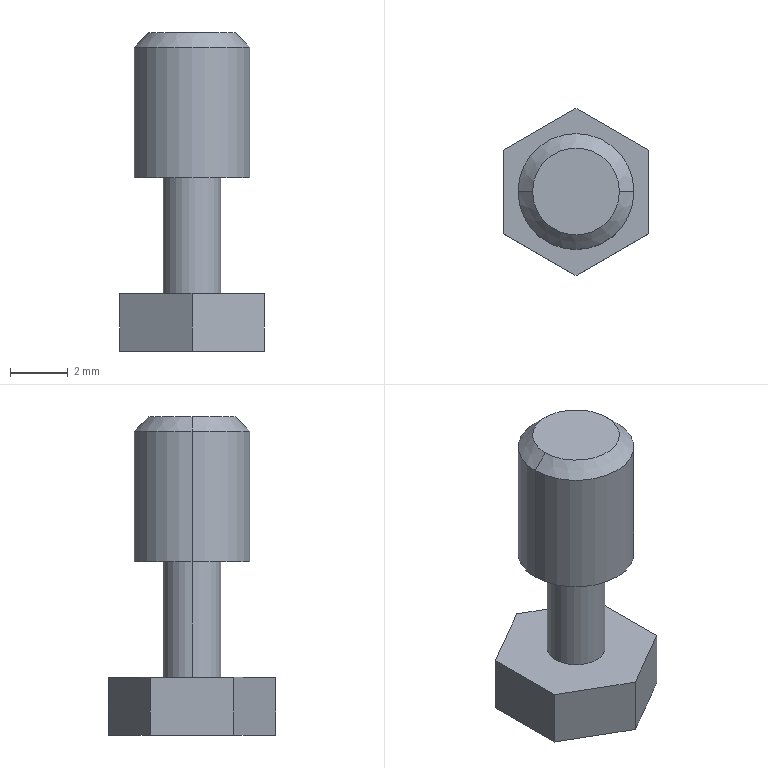Part | SolidWorks | features ICE 2, Chamfer 1, Extrusion 1 | 1 solid | 16 faces | box 5 x 5.774 x 11 mm | volume 117.26 mm3 | plane 10 | cylinder 4 | cone 2 | commonest cylinder face diameters 2 x2 4 x2
STEP:
#1=CARTESIAN_POINT('',(1.5,0.,5.));
#2=VERTEX_POINT('',#1);
#3=CARTESIAN_POINT('',(-1.5,0.,5.));
#4=VERTEX_POINT('',#3);
#5=CARTESIAN_POINT('',(0.,0.,5.));
#6=DIRECTION('',(0.,0.,1.));
#7=DIRECTION('',(1.,0.,0.));
#8=AXIS2_PLACEMENT_3D('',#5,#6,#7);
#9=CIRCLE('',#8,1.5);
#10=EDGE_CURVE('',#2,#4,#9,.T.);
#11=ORIENTED_EDGE('',*,*,#10,.F.);
#12=CARTESIAN_POINT('',(2.,0.,4.5));
#13=VERTEX_POINT('',#12);
#14=CARTESIAN_POINT('',(1.5,0.,5.));
#15=DIRECTION('',(0.7071,0.,-0.7071));
#16=VECTOR('',#15,1000.);
#17=LINE('',#14,#16);
#18=EDGE_CURVE('',#2,#13,#17,.T.);
#19=ORIENTED_EDGE('',*,*,#18,.T.);
#20=CARTESIAN_POINT('',(-2.,0.,4.5));
#21=VERTEX_POINT('',#20);
#22=CARTESIAN_POINT('',(0.,0.,4.5));
#23=DIRECTION('',(0.,0.,-1.));
#24=DIRECTION('',(1.,0.,0.));
#25=AXIS2_PLACEMENT_3D('',#22,#23,#24);
#26=CIRCLE('',#25,2.);
#27=EDGE_CURVE('',#21,#13,#26,.T.);
#28=ORIENTED_EDGE('',*,*,#27,.F.);
#29=CARTESIAN_POINT('',(-1.5,0.,5.));
#30=DIRECTION('',(-0.7071,0.,-0.7071));
#31=VECTOR('',#30,1000.);
#32=LINE('',#29,#31);
#33=EDGE_CURVE('',#4,#21,#32,.T.);
#34=ORIENTED_EDGE('',*,*,#33,.F.);
#35=EDGE_LOOP('',(#11,#19,#28,#34));
#36=FACE_OUTER_BOUND('',#35,.T.);
#37=CARTESIAN_POINT('',(0.,0.,5.));
#38=DIRECTION('',(0.,0.,-1.));
#39=DIRECTION('',(-1.,0.,0.));
#40=AXIS2_PLACEMENT_3D('',#37,#38,#39);
#41=CONICAL_SURFACE('',#40,1.5,0.7854);
#42=ADVANCED_FACE('',(#36),#41,.T.);
#43=CARTESIAN_POINT('',(-1.,0.,-4.));
#44=VERTEX_POINT('',#43);
#45=CARTESIAN_POINT('',(1.,0.,-4.));
#46=VERTEX_POINT('',#45);
#47=CARTESIAN_POINT('',(0.,0.,-4.));
#48=DIRECTION('',(0.,0.,-1.));
#49=DIRECTION('',(-1.,0.,0.));
#50=AXIS2_PLACEMENT_3D('',#47,#48,#49);
#51=CIRCLE('',#50,1.);
#52=EDGE_CURVE('',#44,#46,#51,.T.);
#53=ORIENTED_EDGE('',*,*,#52,.F.);
#54=CARTESIAN_POINT('',(-1.,0.,0.));
#55=VERTEX_POINT('',#54);
#56=CARTESIAN_POINT('',(-1.,0.,-4.));
#57=DIRECTION('',(0.,0.,1.));
#58=VECTOR('',#57,1000.);
#59=LINE('',#56,#58);
#60=EDGE_CURVE('',#44,#55,#59,.T.);
#61=ORIENTED_EDGE('',*,*,#60,.T.);
#62=CARTESIAN_POINT('',(1.,0.,0.));
#63=VERTEX_POINT('',#62);
#64=CARTESIAN_POINT('',(0.,0.,0.));
#65=DIRECTION('',(0.,0.,-1.));
#66=DIRECTION('',(-1.,0.,0.));
#67=AXIS2_PLACEMENT_3D('',#64,#65,#66);
#68=CIRCLE('',#67,1.);
#69=EDGE_CURVE('',#55,#63,#68,.T.);
#70=ORIENTED_EDGE('',*,*,#69,.T.);
#71=CARTESIAN_POINT('',(1.,0.,-4.));
#72=DIRECTION('',(0.,0.,1.));
#73=VECTOR('',#72,1000.);
#74=LINE('',#71,#73);
#75=EDGE_CURVE('',#46,#63,#74,.T.);
#76=ORIENTED_EDGE('',*,*,#75,.F.);
#77=EDGE_LOOP('',(#53,#61,#70,#76));
#78=FACE_OUTER_BOUND('',#77,.T.);
#79=CARTESIAN_POINT('',(0.,0.,-4.));
#80=DIRECTION('',(0.,0.,1.));
#81=DIRECTION('',(1.,0.,0.));
#82=AXIS2_PLACEMENT_3D('',#79,#80,#81);
#83=CYLINDRICAL_SURFACE('',#82,1.);
#84=ADVANCED_FACE('',(#78),#83,.T.);
#85=ORIENTED_EDGE('',*,*,#27,.T.);
#86=CARTESIAN_POINT('',(2.,0.,0.));
#87=VERTEX_POINT('',#86);
#88=CARTESIAN_POINT('',(2.,0.,5.));
#89=DIRECTION('',(0.,0.,-1.));
#90=VECTOR('',#89,1000.);
#91=LINE('',#88,#90);
#92=EDGE_CURVE('',#13,#87,#91,.T.);
#93=ORIENTED_EDGE('',*,*,#92,.T.);
#94=CARTESIAN_POINT('',(-2.,0.,0.));
#95=VERTEX_POINT('',#94);
#96=CARTESIAN_POINT('',(0.,0.,0.));
#97=DIRECTION('',(0.,0.,1.));
#98=DIRECTION('',(1.,0.,0.));
#99=AXIS2_PLACEMENT_3D('',#96,#97,#98);
#100=CIRCLE('',#99,2.);
#101=EDGE_CURVE('',#87,#95,#100,.T.);
#102=ORIENTED_EDGE('',*,*,#101,.T.);
#103=CARTESIAN_POINT('',(-2.,0.,5.));
#104=DIRECTION('',(0.,0.,-1.));
#105=VECTOR('',#104,1000.);
#106=LINE('',#103,#105);
#107=EDGE_CURVE('',#21,#95,#106,.T.);
#108=ORIENTED_EDGE('',*,*,#107,.F.);
#109=EDGE_LOOP('',(#85,#93,#102,#108));
#110=FACE_OUTER_BOUND('',#109,.T.);
#111=CARTESIAN_POINT('',(0.,0.,5.));
#112=DIRECTION('',(0.,0.,-1.));
#113=DIRECTION('',(-1.,0.,0.));
#114=AXIS2_PLACEMENT_3D('',#111,#112,#113);
#115=CYLINDRICAL_SURFACE('',#114,2.);
#116=ADVANCED_FACE('',(#110),#115,.T.);
#117=ORIENTED_EDGE('',*,*,#92,.F.);
#118=CARTESIAN_POINT('',(0.,0.,4.5));
#119=DIRECTION('',(0.,0.,-1.));
#120=DIRECTION('',(1.,0.,0.));
#121=AXIS2_PLACEMENT_3D('',#118,#119,#120);
#122=CIRCLE('',#121,2.);
#123=EDGE_CURVE('',#13,#21,#122,.T.);
#124=ORIENTED_EDGE('',*,*,#123,.T.);
#125=ORIENTED_EDGE('',*,*,#107,.T.);
#126=CARTESIAN_POINT('',(0.,0.,0.));
#127=DIRECTION('',(0.,0.,1.));
#128=DIRECTION('',(1.,0.,0.));
#129=AXIS2_PLACEMENT_3D('',#126,#127,#128);
#130=CIRCLE('',#129,2.);
#131=EDGE_CURVE('',#95,#87,#130,.T.);
#132=ORIENTED_EDGE('',*,*,#131,.T.);
#133=EDGE_LOOP('',(#117,#124,#125,#132));
#134=FACE_OUTER_BOUND('',#133,.T.);
#135=CARTESIAN_POINT('',(0.,0.,5.));
#136=DIRECTION('',(0.,0.,-1.));
#137=DIRECTION('',(-1.,0.,0.));
#138=AXIS2_PLACEMENT_3D('',#135,#136,#137);
#139=CYLINDRICAL_SURFACE('',#138,2.);
#140=ADVANCED_FACE('',(#134),#139,.T.);
#141=CARTESIAN_POINT('',(0.,0.,5.));
#142=DIRECTION('',(0.,0.,1.));
#143=DIRECTION('',(1.,0.,0.));
#144=AXIS2_PLACEMENT_3D('',#141,#142,#143);
#145=CIRCLE('',#144,1.5);
#146=EDGE_CURVE('',#4,#2,#145,.T.);
#147=ORIENTED_EDGE('',*,*,#146,.T.);
#148=ORIENTED_EDGE('',*,*,#10,.T.);
#149=EDGE_LOOP('',(#147,#148));
#150=FACE_OUTER_BOUND('',#149,.T.);
#151=CARTESIAN_POINT('',(0.,0.,5.));
#152=DIRECTION('',(0.,0.,1.));
#153=DIRECTION('',(1.,0.,0.));
#154=AXIS2_PLACEMENT_3D('',#151,#152,#153);
#155=PLANE('',#154);
#156=ADVANCED_FACE('',(#150),#155,.T.);
#157=CARTESIAN_POINT('',(0.,0.,0.));
#158=DIRECTION('',(0.,0.,-1.));
#159=DIRECTION('',(-1.,0.,0.));
#160=AXIS2_PLACEMENT_3D('',#157,#158,#159);
#161=CIRCLE('',#160,1.);
#162=EDGE_CURVE('',#63,#55,#161,.T.);
#163=ORIENTED_EDGE('',*,*,#162,.F.);
#164=ORIENTED_EDGE('',*,*,#69,.F.);
#165=EDGE_LOOP('',(#163,#164));
#166=FACE_BOUND('',#165,.T.);
#167=ORIENTED_EDGE('',*,*,#131,.F.);
#168=ORIENTED_EDGE('',*,*,#101,.F.);
#169=EDGE_LOOP('',(#167,#168));
#170=FACE_OUTER_BOUND('',#169,.T.);
#171=CARTESIAN_POINT('',(0.,0.,0.));
#172=DIRECTION('',(0.,0.,1.));
#173=DIRECTION('',(1.,0.,0.));
#174=AXIS2_PLACEMENT_3D('',#171,#172,#173);
#175=PLANE('',#174);
#176=ADVANCED_FACE('',(#166,#170),#175,.F.);
#177=ORIENTED_EDGE('',*,*,#60,.F.);
#178=CARTESIAN_POINT('',(0.,0.,-4.));
#179=DIRECTION('',(0.,0.,-1.));
#180=DIRECTION('',(-1.,0.,0.));
#181=AXIS2_PLACEMENT_3D('',#178,#179,#180);
#182=CIRCLE('',#181,1.);
#183=EDGE_CURVE('',#46,#44,#182,.T.);
#184=ORIENTED_EDGE('',*,*,#183,.F.);
#185=ORIENTED_EDGE('',*,*,#75,.T.);
#186=ORIENTED_EDGE('',*,*,#162,.T.);
#187=EDGE_LOOP('',(#177,#184,#185,#186));
#188=FACE_OUTER_BOUND('',#187,.T.);
#189=CARTESIAN_POINT('',(0.,0.,-4.));
#190=DIRECTION('',(0.,0.,1.));
#191=DIRECTION('',(1.,0.,0.));
#192=AXIS2_PLACEMENT_3D('',#189,#190,#191);
#193=CYLINDRICAL_SURFACE('',#192,1.);
#194=ADVANCED_FACE('',(#188),#193,.T.);
#195=CARTESIAN_POINT('',(-2.5,1.443,-4.));
#196=VERTEX_POINT('',#195);
#197=CARTESIAN_POINT('',(0.,2.887,-4.));
#198=VERTEX_POINT('',#197);
#199=CARTESIAN_POINT('',(-2.5,1.443,-4.));
#200=DIRECTION('',(0.866,0.5,0.));
#201=VECTOR('',#200,1000.);
#202=LINE('',#199,#201);
#203=EDGE_CURVE('',#196,#198,#202,.T.);
#204=ORIENTED_EDGE('',*,*,#203,.T.);
#205=CARTESIAN_POINT('',(0.,2.887,-6.));
#206=VERTEX_POINT('',#205);
#207=CARTESIAN_POINT('',(0.,2.887,-6.));
#208=DIRECTION('',(0.,0.,1.));
#209=VECTOR('',#208,1000.);
#210=LINE('',#207,#209);
#211=EDGE_CURVE('',#206,#198,#210,.T.);
#212=ORIENTED_EDGE('',*,*,#211,.F.);
#213=CARTESIAN_POINT('',(-2.5,1.443,-6.));
#214=VERTEX_POINT('',#213);
#215=CARTESIAN_POINT('',(-2.5,1.443,-6.));
#216=DIRECTION('',(0.866,0.5,0.));
#217=VECTOR('',#216,1000.);
#218=LINE('',#215,#217);
#219=EDGE_CURVE('',#214,#206,#218,.T.);
#220=ORIENTED_EDGE('',*,*,#219,.F.);
#221=CARTESIAN_POINT('',(-2.5,1.443,-6.));
#222=DIRECTION('',(0.,0.,1.));
#223=VECTOR('',#222,1000.);
#224=LINE('',#221,#223);
#225=EDGE_CURVE('',#214,#196,#224,.T.);
#226=ORIENTED_EDGE('',*,*,#225,.T.);
#227=EDGE_LOOP('',(#204,#212,#220,#226));
#228=FACE_OUTER_BOUND('',#227,.T.);
#229=CARTESIAN_POINT('',(-2.5,1.443,-6.));
#230=DIRECTION('',(0.5,-0.866,0.));
#231=DIRECTION('',(0.866,0.5,0.));
#232=AXIS2_PLACEMENT_3D('',#229,#230,#231);
#233=PLANE('',#232);
#234=ADVANCED_FACE('',(#228),#233,.F.);
#235=CARTESIAN_POINT('',(2.5,1.443,-4.));
#236=VERTEX_POINT('',#235);
#237=CARTESIAN_POINT('',(0.,2.887,-4.));
#238=DIRECTION('',(0.866,-0.5,0.));
#239=VECTOR('',#238,1000.);
#240=LINE('',#237,#239);
#241=EDGE_CURVE('',#198,#236,#240,.T.);
#242=ORIENTED_EDGE('',*,*,#241,.T.);
#243=CARTESIAN_POINT('',(2.5,1.443,-6.));
#244=VERTEX_POINT('',#243);
#245=CARTESIAN_POINT('',(2.5,1.443,-6.));
#246=DIRECTION('',(0.,0.,1.));
#247=VECTOR('',#246,1000.);
#248=LINE('',#245,#247);
#249=EDGE_CURVE('',#244,#236,#248,.T.);
#250=ORIENTED_EDGE('',*,*,#249,.F.);
#251=CARTESIAN_POINT('',(0.,2.887,-6.));
#252=DIRECTION('',(0.866,-0.5,0.));
#253=VECTOR('',#252,1000.);
#254=LINE('',#251,#253);
#255=EDGE_CURVE('',#206,#244,#254,.T.);
#256=ORIENTED_EDGE('',*,*,#255,.F.);
#257=ORIENTED_EDGE('',*,*,#211,.T.);
#258=EDGE_LOOP('',(#242,#250,#256,#257));
#259=FACE_OUTER_BOUND('',#258,.T.);
#260=CARTESIAN_POINT('',(0.,2.887,-6.));
#261=DIRECTION('',(-0.5,-0.866,0.));
#262=DIRECTION('',(0.866,-0.5,0.));
#263=AXIS2_PLACEMENT_3D('',#260,#261,#262);
#264=PLANE('',#263);
#265=ADVANCED_FACE('',(#259),#264,.F.);
#266=CARTESIAN_POINT('',(2.5,-1.443,-4.));
#267=VERTEX_POINT('',#266);
#268=CARTESIAN_POINT('',(2.5,1.443,-4.));
#269=DIRECTION('',(0.,-1.,0.));
#270=VECTOR('',#269,1000.);
#271=LINE('',#268,#270);
#272=EDGE_CURVE('',#236,#267,#271,.T.);
#273=ORIENTED_EDGE('',*,*,#272,.T.);
#274=CARTESIAN_POINT('',(2.5,-1.443,-6.));
#275=VERTEX_POINT('',#274);
#276=CARTESIAN_POINT('',(2.5,-1.443,-6.));
#277=DIRECTION('',(0.,0.,1.));
#278=VECTOR('',#277,1000.);
#279=LINE('',#276,#278);
#280=EDGE_CURVE('',#275,#267,#279,.T.);
#281=ORIENTED_EDGE('',*,*,#280,.F.);
#282=CARTESIAN_POINT('',(2.5,1.443,-6.));
#283=DIRECTION('',(0.,-1.,0.));
#284=VECTOR('',#283,1000.);
#285=LINE('',#282,#284);
#286=EDGE_CURVE('',#244,#275,#285,.T.);
#287=ORIENTED_EDGE('',*,*,#286,.F.);
#288=ORIENTED_EDGE('',*,*,#249,.T.);
#289=EDGE_LOOP('',(#273,#281,#287,#288));
#290=FACE_OUTER_BOUND('',#289,.T.);
#291=CARTESIAN_POINT('',(2.5,1.443,-6.));
#292=DIRECTION('',(-1.,0.,0.));
#293=DIRECTION('',(0.,0.,1.));
#294=AXIS2_PLACEMENT_3D('',#291,#292,#293);
#295=PLANE('',#294);
#296=ADVANCED_FACE('',(#290),#295,.F.);
#297=CARTESIAN_POINT('',(0.,-2.887,-4.));
#298=VERTEX_POINT('',#297);
#299=CARTESIAN_POINT('',(2.5,-1.443,-4.));
#300=DIRECTION('',(-0.866,-0.5,0.));
#301=VECTOR('',#300,1000.);
#302=LINE('',#299,#301);
#303=EDGE_CURVE('',#267,#298,#302,.T.);
#304=ORIENTED_EDGE('',*,*,#303,.T.);
#305=CARTESIAN_POINT('',(0.,-2.887,-6.));
#306=VERTEX_POINT('',#305);
#307=CARTESIAN_POINT('',(0.,-2.887,-6.));
#308=DIRECTION('',(0.,0.,1.));
#309=VECTOR('',#308,1000.);
#310=LINE('',#307,#309);
#311=EDGE_CURVE('',#306,#298,#310,.T.);
#312=ORIENTED_EDGE('',*,*,#311,.F.);
#313=CARTESIAN_POINT('',(2.5,-1.443,-6.));
#314=DIRECTION('',(-0.866,-0.5,0.));
#315=VECTOR('',#314,1000.);
#316=LINE('',#313,#315);
#317=EDGE_CURVE('',#275,#306,#316,.T.);
#318=ORIENTED_EDGE('',*,*,#317,.F.);
#319=ORIENTED_EDGE('',*,*,#280,.T.);
#320=EDGE_LOOP('',(#304,#312,#318,#319));
#321=FACE_OUTER_BOUND('',#320,.T.);
#322=CARTESIAN_POINT('',(2.5,-1.443,-6.));
#323=DIRECTION('',(-0.5,0.866,0.));
#324=DIRECTION('',(-0.866,-0.5,0.));
#325=AXIS2_PLACEMENT_3D('',#322,#323,#324);
#326=PLANE('',#325);
#327=ADVANCED_FACE('',(#321),#326,.F.);
#328=CARTESIAN_POINT('',(-2.5,-1.443,-4.));
#329=VERTEX_POINT('',#328);
#330=CARTESIAN_POINT('',(0.,-2.887,-4.));
#331=DIRECTION('',(-0.866,0.5,0.));
#332=VECTOR('',#331,1000.);
#333=LINE('',#330,#332);
#334=EDGE_CURVE('',#298,#329,#333,.T.);
#335=ORIENTED_EDGE('',*,*,#334,.T.);
#336=CARTESIAN_POINT('',(-2.5,-1.443,-6.));
#337=VERTEX_POINT('',#336);
#338=CARTESIAN_POINT('',(-2.5,-1.443,-6.));
#339=DIRECTION('',(0.,0.,1.));
#340=VECTOR('',#339,1000.);
#341=LINE('',#338,#340);
#342=EDGE_CURVE('',#337,#329,#341,.T.);
#343=ORIENTED_EDGE('',*,*,#342,.F.);
#344=CARTESIAN_POINT('',(0.,-2.887,-6.));
#345=DIRECTION('',(-0.866,0.5,0.));
#346=VECTOR('',#345,1000.);
#347=LINE('',#344,#346);
#348=EDGE_CURVE('',#306,#337,#347,.T.);
#349=ORIENTED_EDGE('',*,*,#348,.F.);
#350=ORIENTED_EDGE('',*,*,#311,.T.);
#351=EDGE_LOOP('',(#335,#343,#349,#350));
#352=FACE_OUTER_BOUND('',#351,.T.);
#353=CARTESIAN_POINT('',(0.,-2.887,-6.));
#354=DIRECTION('',(0.5,0.866,0.));
#355=DIRECTION('',(-0.866,0.5,0.));
#356=AXIS2_PLACEMENT_3D('',#353,#354,#355);
#357=PLANE('',#356);
#358=ADVANCED_FACE('',(#352),#357,.F.);
#359=CARTESIAN_POINT('',(-2.5,-1.443,-4.));
#360=DIRECTION('',(0.,1.,0.));
#361=VECTOR('',#360,1000.);
#362=LINE('',#359,#361);
#363=EDGE_CURVE('',#329,#196,#362,.T.);
#364=ORIENTED_EDGE('',*,*,#363,.T.);
#365=ORIENTED_EDGE('',*,*,#225,.F.);
#366=CARTESIAN_POINT('',(-2.5,-1.443,-6.));
#367=DIRECTION('',(0.,1.,0.));
#368=VECTOR('',#367,1000.);
#369=LINE('',#366,#368);
#370=EDGE_CURVE('',#337,#214,#369,.T.);
#371=ORIENTED_EDGE('',*,*,#370,.F.);
#372=ORIENTED_EDGE('',*,*,#342,.T.);
#373=EDGE_LOOP('',(#364,#365,#371,#372));
#374=FACE_OUTER_BOUND('',#373,.T.);
#375=CARTESIAN_POINT('',(-2.5,-1.443,-6.));
#376=DIRECTION('',(1.,0.,0.));
#377=DIRECTION('',(0.,0.,-1.));
#378=AXIS2_PLACEMENT_3D('',#375,#376,#377);
#379=PLANE('',#378);
#380=ADVANCED_FACE('',(#374),#379,.F.);
#381=ORIENTED_EDGE('',*,*,#219,.T.);
#382=ORIENTED_EDGE('',*,*,#255,.T.);
#383=ORIENTED_EDGE('',*,*,#286,.T.);
#384=ORIENTED_EDGE('',*,*,#317,.T.);
#385=ORIENTED_EDGE('',*,*,#348,.T.);
#386=ORIENTED_EDGE('',*,*,#370,.T.);
#387=EDGE_LOOP('',(#381,#382,#383,#384,#385,#386));
#388=FACE_OUTER_BOUND('',#387,.T.);
#389=CARTESIAN_POINT('',(0.,0.,-6.));
#390=DIRECTION('',(0.,0.,-1.));
#391=DIRECTION('',(-1.,0.,0.));
#392=AXIS2_PLACEMENT_3D('',#389,#390,#391);
#393=PLANE('',#392);
#394=ADVANCED_FACE('',(#388),#393,.T.);
#395=ORIENTED_EDGE('',*,*,#183,.T.);
#396=ORIENTED_EDGE('',*,*,#52,.T.);
#397=EDGE_LOOP('',(#395,#396));
#398=FACE_BOUND('',#397,.T.);
#399=ORIENTED_EDGE('',*,*,#203,.F.);
#400=ORIENTED_EDGE('',*,*,#363,.F.);
#401=ORIENTED_EDGE('',*,*,#334,.F.);
#402=ORIENTED_EDGE('',*,*,#303,.F.);
#403=ORIENTED_EDGE('',*,*,#272,.F.);
#404=ORIENTED_EDGE('',*,*,#241,.F.);
#405=EDGE_LOOP('',(#399,#400,#401,#402,#403,#404));
#406=FACE_OUTER_BOUND('',#405,.T.);
#407=CARTESIAN_POINT('',(0.,0.,-4.));
#408=DIRECTION('',(0.,0.,-1.));
#409=DIRECTION('',(-1.,0.,0.));
#410=AXIS2_PLACEMENT_3D('',#407,#408,#409);
#411=PLANE('',#410);
#412=ADVANCED_FACE('',(#398,#406),#411,.F.);
#413=ORIENTED_EDGE('',*,*,#18,.F.);
#414=ORIENTED_EDGE('',*,*,#146,.F.);
#415=ORIENTED_EDGE('',*,*,#33,.T.);
#416=ORIENTED_EDGE('',*,*,#123,.F.);
#417=EDGE_LOOP('',(#413,#414,#415,#416));
#418=FACE_OUTER_BOUND('',#417,.T.);
#419=CARTESIAN_POINT('',(0.,0.,5.));
#420=DIRECTION('',(0.,0.,-1.));
#421=DIRECTION('',(-1.,0.,0.));
#422=AXIS2_PLACEMENT_3D('',#419,#420,#421);
#423=CONICAL_SURFACE('',#422,1.5,0.7854);
#424=ADVANCED_FACE('',(#418),#423,.T.);
#425=CLOSED_SHELL('',(#42,#84,#116,#140,#156,#176,#194,#234,#265,#296,#327,#358,#380,#394,#412,#424));
#426=MANIFOLD_SOLID_BREP('',#425);
#427=CARTESIAN_POINT('',(0.,0.,0.));
#428=DIRECTION('',(0.,0.,1.));
#429=DIRECTION('',(1.,0.,0.));
#430=AXIS2_PLACEMENT_3D('',#427,#428,#429);
#431=(LENGTH_UNIT()NAMED_UNIT(*)SI_UNIT(.MILLI.,.METRE.));
#432=UNCERTAINTY_MEASURE_WITH_UNIT(LENGTH_MEASURE(0.00001),#431,'','');
#433=(NAMED_UNIT(*)PLANE_ANGLE_UNIT()SI_UNIT($,.RADIAN.));
#434=(NAMED_UNIT(*)SI_UNIT($,.STERADIAN.)SOLID_ANGLE_UNIT());
#435=(GEOMETRIC_REPRESENTATION_CONTEXT(3)GLOBAL_UNCERTAINTY_ASSIGNED_CONTEXT((#432))GLOBAL_UNIT_ASSIGNED_CONTEXT((#431,#433,#434))REPRESENTATION_CONTEXT('',''));
#436=ADVANCED_BREP_SHAPE_REPRESENTATION('',(#426,#430),#435);